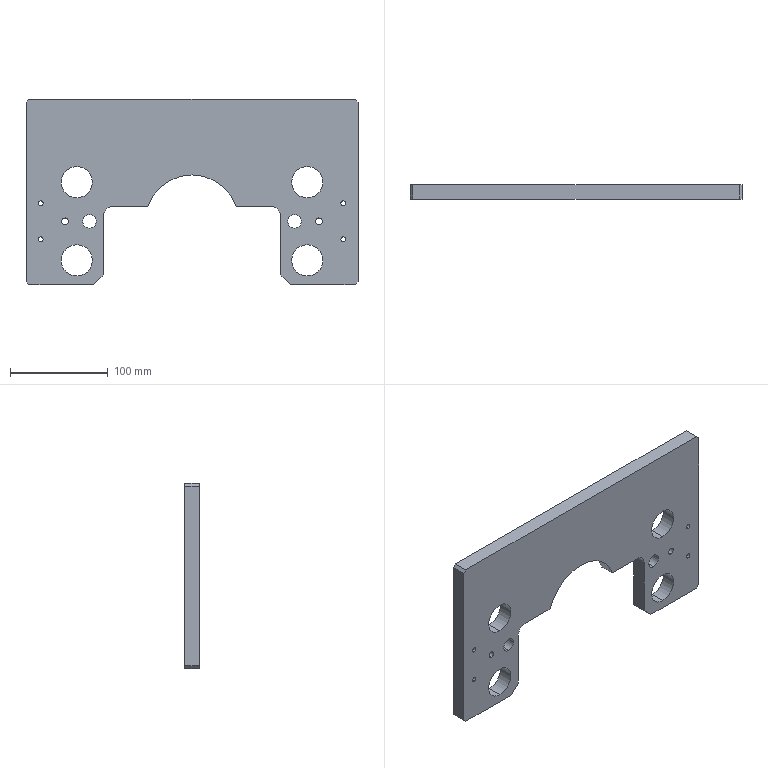Part | STEP file | 227H056238 Middle Base_Default | 1 solid | 45 faces | box 340 x 15 x 190 mm | volume 662186 mm3 | cylinder 28 | plane 17 | commonest cylinder face diameters 5 x8 32 x8 6.8 x4 14 x4 20 x2 95 x2